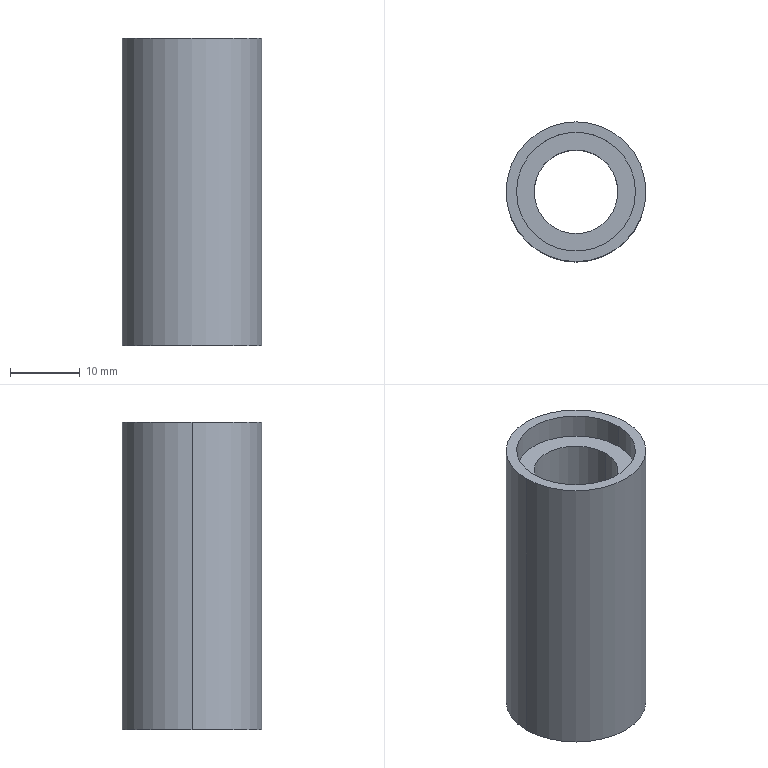Part | STEP file | Shaft 4 PN_0052 | 1 solid | 11 faces | box 20 x 20 x 44 mm | volume 8364 mm3 | cylinder 6 | plane 3 | cone 2 | commonest cylinder face diameters 12 x2 17 x2 20 x2
STEP:
#1=CARTESIAN_POINT('',(0.,0.,0.));
#2=DIRECTION('',(0.,0.,1.));
#3=DIRECTION('',(1.,0.,0.));
#4=AXIS2_PLACEMENT_3D('',#1,#2,#3);
#5=CARTESIAN_POINT('',(10.,0.,0.));
#6=VERTEX_POINT('',#5);
#7=CARTESIAN_POINT('',(-10.,0.,0.));
#8=VERTEX_POINT('',#7);
#9=CARTESIAN_POINT('',(0.,0.,0.));
#10=DIRECTION('',(0.,0.,1.));
#11=DIRECTION('',(1.,0.,0.));
#12=AXIS2_PLACEMENT_3D('',#9,#10,#11);
#13=CIRCLE('',#12,10.);
#14=CARTESIAN_POINT('',(0.,0.,0.));
#15=DIRECTION('',(0.,0.,1.));
#16=DIRECTION('',(1.,0.,0.));
#17=AXIS2_PLACEMENT_3D('',#14,#15,#16);
#18=CYLINDRICAL_SURFACE('',#17,10.);
#19=CARTESIAN_POINT('',(0.,0.));
#20=DIRECTION('',(1.,0.));
#21=VECTOR('',#20,1.);
#22=LINE('',#19,#21);
#23=(GEOMETRIC_REPRESENTATION_CONTEXT(2)PARAMETRIC_REPRESENTATION_CONTEXT()REPRESENTATION_CONTEXT('',''));
#24=DEFINITIONAL_REPRESENTATION('',(#22),#23);
#25=PCURVE('',#18,#24);
#26=CARTESIAN_POINT('',(0.,0.,0.));
#27=DIRECTION('',(0.,0.,-1.));
#28=DIRECTION('',(-1.,0.,0.));
#29=AXIS2_PLACEMENT_3D('',#26,#27,#28);
#30=PLANE('',#29);
#31=CARTESIAN_POINT('',(-10.,0.));
#32=CARTESIAN_POINT('',(-10.,17.321));
#33=CARTESIAN_POINT('',(5.,8.66));
#34=CARTESIAN_POINT('',(20.,0.));
#35=CARTESIAN_POINT('',(5.,-8.66));
#36=CARTESIAN_POINT('',(-10.,-17.321));
#37=CARTESIAN_POINT('',(-10.,0.));
#38=(BOUNDED_CURVE()B_SPLINE_CURVE(2,(#31,#32,#33,#34,#35,#36,#37),.UNSPECIFIED.,.T.,.F.)B_SPLINE_CURVE_WITH_KNOTS((1,2,2,2,2,1),(-2.094,0.,2.094,4.189,6.283,8.378),.UNSPECIFIED.)CURVE()GEOMETRIC_REPRESENTATION_ITEM()RATIONAL_B_SPLINE_CURVE((1.,0.5,1.,0.5,1.,0.5,1.))REPRESENTATION_ITEM(''));
#39=(GEOMETRIC_REPRESENTATION_CONTEXT(2)PARAMETRIC_REPRESENTATION_CONTEXT()REPRESENTATION_CONTEXT('',''));
#40=DEFINITIONAL_REPRESENTATION('',(#38),#39);
#41=PCURVE('',#30,#40);
#42=SURFACE_CURVE('',#13,(#25,#41),.PCURVE_S1.);
#43=EDGE_CURVE('',#6,#8,#42,.T.);
#44=ORIENTED_EDGE('',*,*,#43,.T.);
#45=CARTESIAN_POINT('',(-10.,0.,44.));
#46=VERTEX_POINT('',#45);
#47=CARTESIAN_POINT('',(-10.,0.,0.));
#48=DIRECTION('',(0.,0.,1.));
#49=VECTOR('',#48,1.);
#50=LINE('',#47,#49);
#51=CARTESIAN_POINT('',(3.142,0.));
#52=DIRECTION('',(0.,1.));
#53=VECTOR('',#52,1.);
#54=LINE('',#51,#53);
#55=(GEOMETRIC_REPRESENTATION_CONTEXT(2)PARAMETRIC_REPRESENTATION_CONTEXT()REPRESENTATION_CONTEXT('',''));
#56=DEFINITIONAL_REPRESENTATION('',(#54),#55);
#57=PCURVE('',#18,#56);
#58=CARTESIAN_POINT('',(0.,0.,0.));
#59=DIRECTION('',(0.,0.,1.));
#60=DIRECTION('',(1.,0.,0.));
#61=AXIS2_PLACEMENT_3D('',#58,#59,#60);
#62=CYLINDRICAL_SURFACE('',#61,10.);
#63=CARTESIAN_POINT('',(3.142,0.));
#64=DIRECTION('',(0.,1.));
#65=VECTOR('',#64,1.);
#66=LINE('',#63,#65);
#67=(GEOMETRIC_REPRESENTATION_CONTEXT(2)PARAMETRIC_REPRESENTATION_CONTEXT()REPRESENTATION_CONTEXT('',''));
#68=DEFINITIONAL_REPRESENTATION('',(#66),#67);
#69=PCURVE('',#62,#68);
#70=SURFACE_CURVE('',#50,(#57,#69),.PCURVE_S1.);
#71=EDGE_CURVE('',#8,#46,#70,.T.);
#72=ORIENTED_EDGE('',*,*,#71,.T.);
#73=CARTESIAN_POINT('',(10.,0.,44.));
#74=VERTEX_POINT('',#73);
#75=CARTESIAN_POINT('',(0.,0.,44.));
#76=DIRECTION('',(0.,0.,-1.));
#77=DIRECTION('',(1.,0.,0.));
#78=AXIS2_PLACEMENT_3D('',#75,#76,#77);
#79=CIRCLE('',#78,10.);
#80=CARTESIAN_POINT('',(6.283,44.));
#81=DIRECTION('',(-1.,0.));
#82=VECTOR('',#81,1.);
#83=LINE('',#80,#82);
#84=(GEOMETRIC_REPRESENTATION_CONTEXT(2)PARAMETRIC_REPRESENTATION_CONTEXT()REPRESENTATION_CONTEXT('',''));
#85=DEFINITIONAL_REPRESENTATION('',(#83),#84);
#86=PCURVE('',#18,#85);
#87=CARTESIAN_POINT('',(0.,0.,44.));
#88=DIRECTION('',(0.,0.,-1.));
#89=DIRECTION('',(-1.,0.,0.));
#90=AXIS2_PLACEMENT_3D('',#87,#88,#89);
#91=PLANE('',#90);
#92=CARTESIAN_POINT('',(0.,0.));
#93=DIRECTION('',(-1.,0.));
#94=AXIS2_PLACEMENT_2D('',#92,#93);
#95=CIRCLE('',#94,10.);
#96=(GEOMETRIC_REPRESENTATION_CONTEXT(2)PARAMETRIC_REPRESENTATION_CONTEXT()REPRESENTATION_CONTEXT('',''));
#97=DEFINITIONAL_REPRESENTATION('',(#95),#96);
#98=PCURVE('',#91,#97);
#99=SURFACE_CURVE('',#79,(#86,#98),.PCURVE_S1.);
#100=EDGE_CURVE('',#46,#74,#99,.T.);
#101=ORIENTED_EDGE('',*,*,#100,.T.);
#102=CARTESIAN_POINT('',(10.,0.,0.));
#103=DIRECTION('',(0.,0.,1.));
#104=VECTOR('',#103,1.);
#105=LINE('',#102,#104);
#106=CARTESIAN_POINT('',(0.,0.));
#107=DIRECTION('',(0.,1.));
#108=VECTOR('',#107,1.);
#109=LINE('',#106,#108);
#110=(GEOMETRIC_REPRESENTATION_CONTEXT(2)PARAMETRIC_REPRESENTATION_CONTEXT()REPRESENTATION_CONTEXT('',''));
#111=DEFINITIONAL_REPRESENTATION('',(#109),#110);
#112=PCURVE('',#18,#111);
#113=CARTESIAN_POINT('',(6.283,0.));
#114=DIRECTION('',(0.,1.));
#115=VECTOR('',#114,1.);
#116=LINE('',#113,#115);
#117=(GEOMETRIC_REPRESENTATION_CONTEXT(2)PARAMETRIC_REPRESENTATION_CONTEXT()REPRESENTATION_CONTEXT('',''));
#118=DEFINITIONAL_REPRESENTATION('',(#116),#117);
#119=PCURVE('',#62,#118);
#120=SURFACE_CURVE('',#105,(#112,#119),.PCURVE_S1.);
#121=EDGE_CURVE('',#6,#74,#120,.T.);
#122=ORIENTED_EDGE('',*,*,#121,.F.);
#123=EDGE_LOOP('',(#44,#72,#101,#122));
#124=FACE_BOUND('',#123,.T.);
#125=ADVANCED_FACE('',(#124),#18,.T.);
#126=CARTESIAN_POINT('',(-6.,0.,2.));
#127=VERTEX_POINT('',#126);
#128=CARTESIAN_POINT('',(-8.,0.,-0.000000001));
#129=VERTEX_POINT('',#128);
#130=CARTESIAN_POINT('',(-8.,0.,-0.000000001));
#131=DIRECTION('',(-0.7071,0.,-0.7071));
#132=VECTOR('',#131,1.);
#133=LINE('',#130,#132);
#134=CARTESIAN_POINT('',(0.,0.,-0.000000001));
#135=DIRECTION('',(0.,0.,-1.));
#136=DIRECTION('',(-1.,0.,0.));
#137=AXIS2_PLACEMENT_3D('',#134,#135,#136);
#138=CONICAL_SURFACE('',#137,8.,0.7854);
#139=CARTESIAN_POINT('',(6.283,0.));
#140=DIRECTION('',(0.,1.));
#141=VECTOR('',#140,1.);
#142=LINE('',#139,#141);
#143=(GEOMETRIC_REPRESENTATION_CONTEXT(2)PARAMETRIC_REPRESENTATION_CONTEXT()REPRESENTATION_CONTEXT('',''));
#144=DEFINITIONAL_REPRESENTATION('',(#142),#143);
#145=PCURVE('',#138,#144);
#146=CARTESIAN_POINT('',(0.,0.,-0.000000001));
#147=DIRECTION('',(0.,0.,-1.));
#148=DIRECTION('',(-1.,0.,0.));
#149=AXIS2_PLACEMENT_3D('',#146,#147,#148);
#150=CONICAL_SURFACE('',#149,8.,0.7854);
#151=CARTESIAN_POINT('',(0.,0.));
#152=DIRECTION('',(0.,1.));
#153=VECTOR('',#152,1.);
#154=LINE('',#151,#153);
#155=(GEOMETRIC_REPRESENTATION_CONTEXT(2)PARAMETRIC_REPRESENTATION_CONTEXT()REPRESENTATION_CONTEXT('',''));
#156=DEFINITIONAL_REPRESENTATION('',(#154),#155);
#157=PCURVE('',#150,#156);
#158=SURFACE_CURVE('',#133,(#145,#157),.PCURVE_S1.);
#159=EDGE_CURVE('',#127,#129,#158,.T.);
#160=ORIENTED_EDGE('',*,*,#159,.T.);
#161=CARTESIAN_POINT('',(8.,0.,-0.000000001));
#162=VERTEX_POINT('',#161);
#163=CARTESIAN_POINT('',(0.,0.,-0.000000001));
#164=DIRECTION('',(0.,0.,1.));
#165=DIRECTION('',(-1.,0.,0.));
#166=AXIS2_PLACEMENT_3D('',#163,#164,#165);
#167=CIRCLE('',#166,8.);
#168=CARTESIAN_POINT('',(6.283,0.));
#169=DIRECTION('',(-1.,0.));
#170=VECTOR('',#169,1.);
#171=LINE('',#168,#170);
#172=(GEOMETRIC_REPRESENTATION_CONTEXT(2)PARAMETRIC_REPRESENTATION_CONTEXT()REPRESENTATION_CONTEXT('',''));
#173=DEFINITIONAL_REPRESENTATION('',(#171),#172);
#174=PCURVE('',#138,#173);
#175=CARTESIAN_POINT('',(8.,0.));
#176=CARTESIAN_POINT('',(8.,-13.856));
#177=CARTESIAN_POINT('',(-4.,-6.928));
#178=CARTESIAN_POINT('',(-16.,0.));
#179=CARTESIAN_POINT('',(-4.,6.928));
#180=CARTESIAN_POINT('',(8.,13.856));
#181=CARTESIAN_POINT('',(8.,0.));
#182=(BOUNDED_CURVE()B_SPLINE_CURVE(2,(#175,#176,#177,#178,#179,#180,#181),.UNSPECIFIED.,.T.,.F.)B_SPLINE_CURVE_WITH_KNOTS((1,2,2,2,2,1),(-2.094,0.,2.094,4.189,6.283,8.378),.UNSPECIFIED.)CURVE()GEOMETRIC_REPRESENTATION_ITEM()RATIONAL_B_SPLINE_CURVE((1.,0.5,1.,0.5,1.,0.5,1.))REPRESENTATION_ITEM(''));
#183=(GEOMETRIC_REPRESENTATION_CONTEXT(2)PARAMETRIC_REPRESENTATION_CONTEXT()REPRESENTATION_CONTEXT('',''));
#184=DEFINITIONAL_REPRESENTATION('',(#182),#183);
#185=PCURVE('',#30,#184);
#186=SURFACE_CURVE('',#167,(#174,#185),.PCURVE_S1.);
#187=EDGE_CURVE('',#129,#162,#186,.T.);
#188=ORIENTED_EDGE('',*,*,#187,.T.);
#189=CARTESIAN_POINT('',(6.,0.,2.));
#190=VERTEX_POINT('',#189);
#191=CARTESIAN_POINT('',(8.,0.,-0.000000001));
#192=DIRECTION('',(0.7071,0.,-0.7071));
#193=VECTOR('',#192,1.);
#194=LINE('',#191,#193);
#195=CARTESIAN_POINT('',(3.142,0.));
#196=DIRECTION('',(0.,1.));
#197=VECTOR('',#196,1.);
#198=LINE('',#195,#197);
#199=(GEOMETRIC_REPRESENTATION_CONTEXT(2)PARAMETRIC_REPRESENTATION_CONTEXT()REPRESENTATION_CONTEXT('',''));
#200=DEFINITIONAL_REPRESENTATION('',(#198),#199);
#201=PCURVE('',#138,#200);
#202=CARTESIAN_POINT('',(3.142,0.));
#203=DIRECTION('',(0.,1.));
#204=VECTOR('',#203,1.);
#205=LINE('',#202,#204);
#206=(GEOMETRIC_REPRESENTATION_CONTEXT(2)PARAMETRIC_REPRESENTATION_CONTEXT()REPRESENTATION_CONTEXT('',''));
#207=DEFINITIONAL_REPRESENTATION('',(#205),#206);
#208=PCURVE('',#150,#207);
#209=SURFACE_CURVE('',#194,(#201,#208),.PCURVE_S1.);
#210=EDGE_CURVE('',#190,#162,#209,.T.);
#211=ORIENTED_EDGE('',*,*,#210,.F.);
#212=CARTESIAN_POINT('',(0.,0.,2.));
#213=DIRECTION('',(0.,0.,-1.));
#214=DIRECTION('',(1.,0.,0.));
#215=AXIS2_PLACEMENT_3D('',#212,#213,#214);
#216=CIRCLE('',#215,6.);
#217=CARTESIAN_POINT('',(3.142,-2.));
#218=DIRECTION('',(1.,0.));
#219=VECTOR('',#218,1.);
#220=LINE('',#217,#219);
#221=(GEOMETRIC_REPRESENTATION_CONTEXT(2)PARAMETRIC_REPRESENTATION_CONTEXT()REPRESENTATION_CONTEXT('',''));
#222=DEFINITIONAL_REPRESENTATION('',(#220),#221);
#223=PCURVE('',#138,#222);
#224=CARTESIAN_POINT('',(0.,0.,0.));
#225=DIRECTION('',(0.,0.,1.));
#226=DIRECTION('',(1.,0.,0.));
#227=AXIS2_PLACEMENT_3D('',#224,#225,#226);
#228=CYLINDRICAL_SURFACE('',#227,6.);
#229=CARTESIAN_POINT('',(6.283,2.));
#230=DIRECTION('',(-1.,0.));
#231=VECTOR('',#230,1.);
#232=LINE('',#229,#231);
#233=(GEOMETRIC_REPRESENTATION_CONTEXT(2)PARAMETRIC_REPRESENTATION_CONTEXT()REPRESENTATION_CONTEXT('',''));
#234=DEFINITIONAL_REPRESENTATION('',(#232),#233);
#235=PCURVE('',#228,#234);
#236=SURFACE_CURVE('',#216,(#223,#235),.PCURVE_S1.);
#237=EDGE_CURVE('',#190,#127,#236,.T.);
#238=ORIENTED_EDGE('',*,*,#237,.T.);
#239=EDGE_LOOP('',(#160,#188,#211,#238));
#240=FACE_BOUND('',#239,.F.);
#241=ADVANCED_FACE('',(#240),#138,.F.);
#242=CARTESIAN_POINT('',(-8.5,0.,44.));
#243=VERTEX_POINT('',#242);
#244=CARTESIAN_POINT('',(-8.5,0.,40.5));
#245=VERTEX_POINT('',#244);
#246=CARTESIAN_POINT('',(-8.5,0.,44.));
#247=DIRECTION('',(0.,0.,-1.));
#248=VECTOR('',#247,1.);
#249=LINE('',#246,#248);
#250=CARTESIAN_POINT('',(0.,0.,44.));
#251=DIRECTION('',(0.,0.,-1.));
#252=DIRECTION('',(-1.,0.,0.));
#253=AXIS2_PLACEMENT_3D('',#250,#251,#252);
#254=CYLINDRICAL_SURFACE('',#253,8.5);
#255=CARTESIAN_POINT('',(6.283,0.));
#256=DIRECTION('',(0.,1.));
#257=VECTOR('',#256,1.);
#258=LINE('',#255,#257);
#259=(GEOMETRIC_REPRESENTATION_CONTEXT(2)PARAMETRIC_REPRESENTATION_CONTEXT()REPRESENTATION_CONTEXT('',''));
#260=DEFINITIONAL_REPRESENTATION('',(#258),#259);
#261=PCURVE('',#254,#260);
#262=CARTESIAN_POINT('',(0.,0.,44.));
#263=DIRECTION('',(0.,0.,-1.));
#264=DIRECTION('',(-1.,0.,0.));
#265=AXIS2_PLACEMENT_3D('',#262,#263,#264);
#266=CYLINDRICAL_SURFACE('',#265,8.5);
#267=CARTESIAN_POINT('',(0.,0.));
#268=DIRECTION('',(0.,1.));
#269=VECTOR('',#268,1.);
#270=LINE('',#267,#269);
#271=(GEOMETRIC_REPRESENTATION_CONTEXT(2)PARAMETRIC_REPRESENTATION_CONTEXT()REPRESENTATION_CONTEXT('',''));
#272=DEFINITIONAL_REPRESENTATION('',(#270),#271);
#273=PCURVE('',#266,#272);
#274=SURFACE_CURVE('',#249,(#261,#273),.PCURVE_S1.);
#275=EDGE_CURVE('',#243,#245,#274,.T.);
#276=ORIENTED_EDGE('',*,*,#275,.T.);
#277=CARTESIAN_POINT('',(8.5,0.,40.5));
#278=VERTEX_POINT('',#277);
#279=CARTESIAN_POINT('',(0.,0.,40.5));
#280=DIRECTION('',(0.,0.,1.));
#281=DIRECTION('',(-1.,0.,0.));
#282=AXIS2_PLACEMENT_3D('',#279,#280,#281);
#283=CIRCLE('',#282,8.5);
#284=CARTESIAN_POINT('',(6.283,3.5));
#285=DIRECTION('',(-1.,0.));
#286=VECTOR('',#285,1.);
#287=LINE('',#284,#286);
#288=(GEOMETRIC_REPRESENTATION_CONTEXT(2)PARAMETRIC_REPRESENTATION_CONTEXT()REPRESENTATION_CONTEXT('',''));
#289=DEFINITIONAL_REPRESENTATION('',(#287),#288);
#290=PCURVE('',#254,#289);
#291=CARTESIAN_POINT('',(0.,0.,40.5));
#292=DIRECTION('',(0.,0.,-1.));
#293=DIRECTION('',(-1.,0.,0.));
#294=AXIS2_PLACEMENT_3D('',#291,#292,#293);
#295=PLANE('',#294);
#296=CARTESIAN_POINT('',(8.5,0.));
#297=CARTESIAN_POINT('',(8.5,-14.722));
#298=CARTESIAN_POINT('',(-4.25,-7.361));
#299=CARTESIAN_POINT('',(-17.,0.));
#300=CARTESIAN_POINT('',(-4.25,7.361));
#301=CARTESIAN_POINT('',(8.5,14.722));
#302=CARTESIAN_POINT('',(8.5,0.));
#303=(BOUNDED_CURVE()B_SPLINE_CURVE(2,(#296,#297,#298,#299,#300,#301,#302),.UNSPECIFIED.,.T.,.F.)B_SPLINE_CURVE_WITH_KNOTS((1,2,2,2,2,1),(-2.094,0.,2.094,4.189,6.283,8.378),.UNSPECIFIED.)CURVE()GEOMETRIC_REPRESENTATION_ITEM()RATIONAL_B_SPLINE_CURVE((1.,0.5,1.,0.5,1.,0.5,1.))REPRESENTATION_ITEM(''));
#304=(GEOMETRIC_REPRESENTATION_CONTEXT(2)PARAMETRIC_REPRESENTATION_CONTEXT()REPRESENTATION_CONTEXT('',''));
#305=DEFINITIONAL_REPRESENTATION('',(#303),#304);
#306=PCURVE('',#295,#305);
#307=SURFACE_CURVE('',#283,(#290,#306),.PCURVE_S1.);
#308=EDGE_CURVE('',#245,#278,#307,.T.);
#309=ORIENTED_EDGE('',*,*,#308,.T.);
#310=CARTESIAN_POINT('',(8.5,0.,44.));
#311=VERTEX_POINT('',#310);
#312=CARTESIAN_POINT('',(8.5,0.,44.));
#313=DIRECTION('',(0.,0.,-1.));
#314=VECTOR('',#313,1.);
#315=LINE('',#312,#314);
#316=CARTESIAN_POINT('',(3.142,0.));
#317=DIRECTION('',(0.,1.));
#318=VECTOR('',#317,1.);
#319=LINE('',#316,#318);
#320=(GEOMETRIC_REPRESENTATION_CONTEXT(2)PARAMETRIC_REPRESENTATION_CONTEXT()REPRESENTATION_CONTEXT('',''));
#321=DEFINITIONAL_REPRESENTATION('',(#319),#320);
#322=PCURVE('',#254,#321);
#323=CARTESIAN_POINT('',(3.142,0.));
#324=DIRECTION('',(0.,1.));
#325=VECTOR('',#324,1.);
#326=LINE('',#323,#325);
#327=(GEOMETRIC_REPRESENTATION_CONTEXT(2)PARAMETRIC_REPRESENTATION_CONTEXT()REPRESENTATION_CONTEXT('',''));
#328=DEFINITIONAL_REPRESENTATION('',(#326),#327);
#329=PCURVE('',#266,#328);
#330=SURFACE_CURVE('',#315,(#322,#329),.PCURVE_S1.);
#331=EDGE_CURVE('',#311,#278,#330,.T.);
#332=ORIENTED_EDGE('',*,*,#331,.F.);
#333=CARTESIAN_POINT('',(0.,0.,44.));
#334=DIRECTION('',(0.,0.,1.));
#335=DIRECTION('',(-1.,0.,0.));
#336=AXIS2_PLACEMENT_3D('',#333,#334,#335);
#337=CIRCLE('',#336,8.5);
#338=CARTESIAN_POINT('',(6.283,0.));
#339=DIRECTION('',(-1.,0.));
#340=VECTOR('',#339,1.);
#341=LINE('',#338,#340);
#342=(GEOMETRIC_REPRESENTATION_CONTEXT(2)PARAMETRIC_REPRESENTATION_CONTEXT()REPRESENTATION_CONTEXT('',''));
#343=DEFINITIONAL_REPRESENTATION('',(#341),#342);
#344=PCURVE('',#254,#343);
#345=CARTESIAN_POINT('',(8.5,0.));
#346=CARTESIAN_POINT('',(8.5,-14.722));
#347=CARTESIAN_POINT('',(-4.25,-7.361));
#348=CARTESIAN_POINT('',(-17.,0.));
#349=CARTESIAN_POINT('',(-4.25,7.361));
#350=CARTESIAN_POINT('',(8.5,14.722));
#351=CARTESIAN_POINT('',(8.5,0.));
#352=(BOUNDED_CURVE()B_SPLINE_CURVE(2,(#345,#346,#347,#348,#349,#350,#351),.UNSPECIFIED.,.T.,.F.)B_SPLINE_CURVE_WITH_KNOTS((1,2,2,2,2,1),(-2.094,0.,2.094,4.189,6.283,8.378),.UNSPECIFIED.)CURVE()GEOMETRIC_REPRESENTATION_ITEM()RATIONAL_B_SPLINE_CURVE((1.,0.5,1.,0.5,1.,0.5,1.))REPRESENTATION_ITEM(''));
#353=(GEOMETRIC_REPRESENTATION_CONTEXT(2)PARAMETRIC_REPRESENTATION_CONTEXT()REPRESENTATION_CONTEXT('',''));
#354=DEFINITIONAL_REPRESENTATION('',(#352),#353);
#355=PCURVE('',#91,#354);
#356=SURFACE_CURVE('',#337,(#344,#355),.PCURVE_S1.);
#357=EDGE_CURVE('',#243,#311,#356,.T.);
#358=ORIENTED_EDGE('',*,*,#357,.F.);
#359=EDGE_LOOP('',(#276,#309,#332,#358));
#360=FACE_BOUND('',#359,.F.);
#361=ADVANCED_FACE('',(#360),#254,.F.);
#362=CARTESIAN_POINT('',(6.,0.,40.5));
#363=VERTEX_POINT('',#362);
#364=CARTESIAN_POINT('',(6.,0.,0.));
#365=DIRECTION('',(0.,0.,1.));
#366=VECTOR('',#365,1.);
#367=LINE('',#364,#366);
#368=CARTESIAN_POINT('',(6.283,0.));
#369=DIRECTION('',(0.,1.));
#370=VECTOR('',#369,1.);
#371=LINE('',#368,#370);
#372=(GEOMETRIC_REPRESENTATION_CONTEXT(2)PARAMETRIC_REPRESENTATION_CONTEXT()REPRESENTATION_CONTEXT('',''));
#373=DEFINITIONAL_REPRESENTATION('',(#371),#372);
#374=PCURVE('',#228,#373);
#375=CARTESIAN_POINT('',(0.,0.,0.));
#376=DIRECTION('',(0.,0.,1.));
#377=DIRECTION('',(1.,0.,0.));
#378=AXIS2_PLACEMENT_3D('',#375,#376,#377);
#379=CYLINDRICAL_SURFACE('',#378,6.);
#380=CARTESIAN_POINT('',(0.,0.));
#381=DIRECTION('',(0.,1.));
#382=VECTOR('',#381,1.);
#383=LINE('',#380,#382);
#384=(GEOMETRIC_REPRESENTATION_CONTEXT(2)PARAMETRIC_REPRESENTATION_CONTEXT()REPRESENTATION_CONTEXT('',''));
#385=DEFINITIONAL_REPRESENTATION('',(#383),#384);
#386=PCURVE('',#379,#385);
#387=SURFACE_CURVE('',#367,(#374,#386),.PCURVE_S1.);
#388=EDGE_CURVE('',#190,#363,#387,.T.);
#389=ORIENTED_EDGE('',*,*,#388,.T.);
#390=CARTESIAN_POINT('',(-6.,0.,40.5));
#391=VERTEX_POINT('',#390);
#392=CARTESIAN_POINT('',(0.,0.,40.5));
#393=DIRECTION('',(0.,0.,-1.));
#394=DIRECTION('',(1.,0.,0.));
#395=AXIS2_PLACEMENT_3D('',#392,#393,#394);
#396=CIRCLE('',#395,6.);
#397=CARTESIAN_POINT('',(6.283,40.5));
#398=DIRECTION('',(-1.,0.));
#399=VECTOR('',#398,1.);
#400=LINE('',#397,#399);
#401=(GEOMETRIC_REPRESENTATION_CONTEXT(2)PARAMETRIC_REPRESENTATION_CONTEXT()REPRESENTATION_CONTEXT('',''));
#402=DEFINITIONAL_REPRESENTATION('',(#400),#401);
#403=PCURVE('',#228,#402);
#404=CARTESIAN_POINT('',(0.,0.));
#405=DIRECTION('',(-1.,0.));
#406=AXIS2_PLACEMENT_2D('',#404,#405);
#407=CIRCLE('',#406,6.);
#408=(GEOMETRIC_REPRESENTATION_CONTEXT(2)PARAMETRIC_REPRESENTATION_CONTEXT()REPRESENTATION_CONTEXT('',''));
#409=DEFINITIONAL_REPRESENTATION('',(#407),#408);
#410=PCURVE('',#295,#409);
#411=SURFACE_CURVE('',#396,(#403,#410),.PCURVE_S1.);
#412=EDGE_CURVE('',#363,#391,#411,.T.);
#413=ORIENTED_EDGE('',*,*,#412,.T.);
#414=CARTESIAN_POINT('',(-6.,0.,0.));
#415=DIRECTION('',(0.,0.,1.));
#416=VECTOR('',#415,1.);
#417=LINE('',#414,#416);
#418=CARTESIAN_POINT('',(3.142,0.));
#419=DIRECTION('',(0.,1.));
#420=VECTOR('',#419,1.);
#421=LINE('',#418,#420);
#422=(GEOMETRIC_REPRESENTATION_CONTEXT(2)PARAMETRIC_REPRESENTATION_CONTEXT()REPRESENTATION_CONTEXT('',''));
#423=DEFINITIONAL_REPRESENTATION('',(#421),#422);
#424=PCURVE('',#228,#423);
#425=CARTESIAN_POINT('',(3.142,0.));
#426=DIRECTION('',(0.,1.));
#427=VECTOR('',#426,1.);
#428=LINE('',#425,#427);
#429=(GEOMETRIC_REPRESENTATION_CONTEXT(2)PARAMETRIC_REPRESENTATION_CONTEXT()REPRESENTATION_CONTEXT('',''));
#430=DEFINITIONAL_REPRESENTATION('',(#428),#429);
#431=PCURVE('',#379,#430);
#432=SURFACE_CURVE('',#417,(#424,#431),.PCURVE_S1.);
#433=EDGE_CURVE('',#127,#391,#432,.T.);
#434=ORIENTED_EDGE('',*,*,#433,.F.);
#435=ORIENTED_EDGE('',*,*,#237,.F.);
#436=EDGE_LOOP('',(#389,#413,#434,#435));
#437=FACE_BOUND('',#436,.F.);
#438=ADVANCED_FACE('',(#437),#228,.F.);
#439=ORIENTED_EDGE('',*,*,#71,.F.);
#440=CARTESIAN_POINT('',(0.,0.,0.));
#441=DIRECTION('',(0.,0.,1.));
#442=DIRECTION('',(1.,0.,0.));
#443=AXIS2_PLACEMENT_3D('',#440,#441,#442);
#444=CIRCLE('',#443,10.);
#445=CARTESIAN_POINT('',(0.,0.));
#446=DIRECTION('',(1.,0.));
#447=VECTOR('',#446,1.);
#448=LINE('',#445,#447);
#449=(GEOMETRIC_REPRESENTATION_CONTEXT(2)PARAMETRIC_REPRESENTATION_CONTEXT()REPRESENTATION_CONTEXT('',''));
#450=DEFINITIONAL_REPRESENTATION('',(#448),#449);
#451=PCURVE('',#62,#450);
#452=CARTESIAN_POINT('',(-10.,0.));
#453=CARTESIAN_POINT('',(-10.,17.321));
#454=CARTESIAN_POINT('',(5.,8.66));
#455=CARTESIAN_POINT('',(20.,0.));
#456=CARTESIAN_POINT('',(5.,-8.66));
#457=CARTESIAN_POINT('',(-10.,-17.321));
#458=CARTESIAN_POINT('',(-10.,0.));
#459=(BOUNDED_CURVE()B_SPLINE_CURVE(2,(#452,#453,#454,#455,#456,#457,#458),.UNSPECIFIED.,.T.,.F.)B_SPLINE_CURVE_WITH_KNOTS((1,2,2,2,2,1),(-2.094,0.,2.094,4.189,6.283,8.378),.UNSPECIFIED.)CURVE()GEOMETRIC_REPRESENTATION_ITEM()RATIONAL_B_SPLINE_CURVE((1.,0.5,1.,0.5,1.,0.5,1.))REPRESENTATION_ITEM(''));
#460=(GEOMETRIC_REPRESENTATION_CONTEXT(2)PARAMETRIC_REPRESENTATION_CONTEXT()REPRESENTATION_CONTEXT('',''));
#461=DEFINITIONAL_REPRESENTATION('',(#459),#460);
#462=PCURVE('',#30,#461);
#463=SURFACE_CURVE('',#444,(#451,#462),.PCURVE_S1.);
#464=EDGE_CURVE('',#8,#6,#463,.T.);
#465=ORIENTED_EDGE('',*,*,#464,.T.);
#466=ORIENTED_EDGE('',*,*,#121,.T.);
#467=CARTESIAN_POINT('',(0.,0.,44.));
#468=DIRECTION('',(0.,0.,-1.));
#469=DIRECTION('',(1.,0.,0.));
#470=AXIS2_PLACEMENT_3D('',#467,#468,#469);
#471=CIRCLE('',#470,10.);
#472=CARTESIAN_POINT('',(6.283,44.));
#473=DIRECTION('',(-1.,0.));
#474=VECTOR('',#473,1.);
#475=LINE('',#472,#474);
#476=(GEOMETRIC_REPRESENTATION_CONTEXT(2)PARAMETRIC_REPRESENTATION_CONTEXT()REPRESENTATION_CONTEXT('',''));
#477=DEFINITIONAL_REPRESENTATION('',(#475),#476);
#478=PCURVE('',#62,#477);
#479=CARTESIAN_POINT('',(0.,0.));
#480=DIRECTION('',(-1.,0.));
#481=AXIS2_PLACEMENT_2D('',#479,#480);
#482=CIRCLE('',#481,10.);
#483=(GEOMETRIC_REPRESENTATION_CONTEXT(2)PARAMETRIC_REPRESENTATION_CONTEXT()REPRESENTATION_CONTEXT('',''));
#484=DEFINITIONAL_REPRESENTATION('',(#482),#483);
#485=PCURVE('',#91,#484);
#486=SURFACE_CURVE('',#471,(#478,#485),.PCURVE_S1.);
#487=EDGE_CURVE('',#74,#46,#486,.T.);
#488=ORIENTED_EDGE('',*,*,#487,.T.);
#489=EDGE_LOOP('',(#439,#465,#466,#488));
#490=FACE_BOUND('',#489,.T.);
#491=ADVANCED_FACE('',(#490),#62,.T.);
#492=ORIENTED_EDGE('',*,*,#187,.T.);
#493=CARTESIAN_POINT('',(0.,0.,-0.000000001));
#494=DIRECTION('',(0.,0.,1.));
#495=DIRECTION('',(-1.,0.,0.));
#496=AXIS2_PLACEMENT_3D('',#493,#494,#495);
#497=CIRCLE('',#496,8.);
#498=CARTESIAN_POINT('',(8.,0.));
#499=CARTESIAN_POINT('',(8.,-13.856));
#500=CARTESIAN_POINT('',(-4.,-6.928));
#501=CARTESIAN_POINT('',(-16.,0.));
#502=CARTESIAN_POINT('',(-4.,6.928));
#503=CARTESIAN_POINT('',(8.,13.856));
#504=CARTESIAN_POINT('',(8.,0.));
#505=(BOUNDED_CURVE()B_SPLINE_CURVE(2,(#498,#499,#500,#501,#502,#503,#504),.UNSPECIFIED.,.T.,.F.)B_SPLINE_CURVE_WITH_KNOTS((1,2,2,2,2,1),(-2.094,0.,2.094,4.189,6.283,8.378),.UNSPECIFIED.)CURVE()GEOMETRIC_REPRESENTATION_ITEM()RATIONAL_B_SPLINE_CURVE((1.,0.5,1.,0.5,1.,0.5,1.))REPRESENTATION_ITEM(''));
#506=(GEOMETRIC_REPRESENTATION_CONTEXT(2)PARAMETRIC_REPRESENTATION_CONTEXT()REPRESENTATION_CONTEXT('',''));
#507=DEFINITIONAL_REPRESENTATION('',(#505),#506);
#508=PCURVE('',#30,#507);
#509=CARTESIAN_POINT('',(6.283,0.));
#510=DIRECTION('',(-1.,0.));
#511=VECTOR('',#510,1.);
#512=LINE('',#509,#511);
#513=(GEOMETRIC_REPRESENTATION_CONTEXT(2)PARAMETRIC_REPRESENTATION_CONTEXT()REPRESENTATION_CONTEXT('',''));
#514=DEFINITIONAL_REPRESENTATION('',(#512),#513);
#515=PCURVE('',#150,#514);
#516=SURFACE_CURVE('',#497,(#508,#515),.PCURVE_S1.);
#517=EDGE_CURVE('',#162,#129,#516,.T.);
#518=ORIENTED_EDGE('',*,*,#517,.T.);
#519=EDGE_LOOP('',(#492,#518));
#520=FACE_BOUND('',#519,.T.);
#521=ORIENTED_EDGE('',*,*,#43,.F.);
#522=ORIENTED_EDGE('',*,*,#464,.F.);
#523=EDGE_LOOP('',(#521,#522));
#524=FACE_BOUND('',#523,.T.);
#525=ADVANCED_FACE('',(#520,#524),#30,.T.);
#526=ORIENTED_EDGE('',*,*,#357,.F.);
#527=CARTESIAN_POINT('',(0.,0.,44.));
#528=DIRECTION('',(0.,0.,1.));
#529=DIRECTION('',(-1.,0.,0.));
#530=AXIS2_PLACEMENT_3D('',#527,#528,#529);
#531=CIRCLE('',#530,8.5);
#532=CARTESIAN_POINT('',(8.5,0.));
#533=CARTESIAN_POINT('',(8.5,-14.722));
#534=CARTESIAN_POINT('',(-4.25,-7.361));
#535=CARTESIAN_POINT('',(-17.,0.));
#536=CARTESIAN_POINT('',(-4.25,7.361));
#537=CARTESIAN_POINT('',(8.5,14.722));
#538=CARTESIAN_POINT('',(8.5,0.));
#539=(BOUNDED_CURVE()B_SPLINE_CURVE(2,(#532,#533,#534,#535,#536,#537,#538),.UNSPECIFIED.,.T.,.F.)B_SPLINE_CURVE_WITH_KNOTS((1,2,2,2,2,1),(-2.094,0.,2.094,4.189,6.283,8.378),.UNSPECIFIED.)CURVE()GEOMETRIC_REPRESENTATION_ITEM()RATIONAL_B_SPLINE_CURVE((1.,0.5,1.,0.5,1.,0.5,1.))REPRESENTATION_ITEM(''));
#540=(GEOMETRIC_REPRESENTATION_CONTEXT(2)PARAMETRIC_REPRESENTATION_CONTEXT()REPRESENTATION_CONTEXT('',''));
#541=DEFINITIONAL_REPRESENTATION('',(#539),#540);
#542=PCURVE('',#91,#541);
#543=CARTESIAN_POINT('',(6.283,0.));
#544=DIRECTION('',(-1.,0.));
#545=VECTOR('',#544,1.);
#546=LINE('',#543,#545);
#547=(GEOMETRIC_REPRESENTATION_CONTEXT(2)PARAMETRIC_REPRESENTATION_CONTEXT()REPRESENTATION_CONTEXT('',''));
#548=DEFINITIONAL_REPRESENTATION('',(#546),#547);
#549=PCURVE('',#266,#548);
#550=SURFACE_CURVE('',#531,(#542,#549),.PCURVE_S1.);
#551=EDGE_CURVE('',#311,#243,#550,.T.);
#552=ORIENTED_EDGE('',*,*,#551,.F.);
#553=EDGE_LOOP('',(#526,#552));
#554=FACE_BOUND('',#553,.T.);
#555=ORIENTED_EDGE('',*,*,#487,.F.);
#556=ORIENTED_EDGE('',*,*,#100,.F.);
#557=EDGE_LOOP('',(#555,#556));
#558=FACE_BOUND('',#557,.T.);
#559=ADVANCED_FACE('',(#554,#558),#91,.F.);
#560=ORIENTED_EDGE('',*,*,#517,.T.);
#561=ORIENTED_EDGE('',*,*,#159,.F.);
#562=CARTESIAN_POINT('',(0.,0.,2.));
#563=DIRECTION('',(0.,0.,-1.));
#564=DIRECTION('',(1.,0.,0.));
#565=AXIS2_PLACEMENT_3D('',#562,#563,#564);
#566=CIRCLE('',#565,6.);
#567=CARTESIAN_POINT('',(-3.142,-2.));
#568=DIRECTION('',(1.,0.));
#569=VECTOR('',#568,1.);
#570=LINE('',#567,#569);
#571=(GEOMETRIC_REPRESENTATION_CONTEXT(2)PARAMETRIC_REPRESENTATION_CONTEXT()REPRESENTATION_CONTEXT('',''));
#572=DEFINITIONAL_REPRESENTATION('',(#570),#571);
#573=PCURVE('',#150,#572);
#574=CARTESIAN_POINT('',(6.283,2.));
#575=DIRECTION('',(-1.,0.));
#576=VECTOR('',#575,1.);
#577=LINE('',#574,#576);
#578=(GEOMETRIC_REPRESENTATION_CONTEXT(2)PARAMETRIC_REPRESENTATION_CONTEXT()REPRESENTATION_CONTEXT('',''));
#579=DEFINITIONAL_REPRESENTATION('',(#577),#578);
#580=PCURVE('',#379,#579);
#581=SURFACE_CURVE('',#566,(#573,#580),.PCURVE_S1.);
#582=EDGE_CURVE('',#127,#190,#581,.T.);
#583=ORIENTED_EDGE('',*,*,#582,.T.);
#584=ORIENTED_EDGE('',*,*,#210,.T.);
#585=EDGE_LOOP('',(#560,#561,#583,#584));
#586=FACE_BOUND('',#585,.F.);
#587=ADVANCED_FACE('',(#586),#150,.F.);
#588=CARTESIAN_POINT('',(0.,0.,40.5));
#589=DIRECTION('',(0.,0.,1.));
#590=DIRECTION('',(-1.,0.,0.));
#591=AXIS2_PLACEMENT_3D('',#588,#589,#590);
#592=CIRCLE('',#591,8.5);
#593=CARTESIAN_POINT('',(6.283,3.5));
#594=DIRECTION('',(-1.,0.));
#595=VECTOR('',#594,1.);
#596=LINE('',#593,#595);
#597=(GEOMETRIC_REPRESENTATION_CONTEXT(2)PARAMETRIC_REPRESENTATION_CONTEXT()REPRESENTATION_CONTEXT('',''));
#598=DEFINITIONAL_REPRESENTATION('',(#596),#597);
#599=PCURVE('',#266,#598);
#600=CARTESIAN_POINT('',(8.5,0.));
#601=CARTESIAN_POINT('',(8.5,-14.722));
#602=CARTESIAN_POINT('',(-4.25,-7.361));
#603=CARTESIAN_POINT('',(-17.,0.));
#604=CARTESIAN_POINT('',(-4.25,7.361));
#605=CARTESIAN_POINT('',(8.5,14.722));
#606=CARTESIAN_POINT('',(8.5,0.));
#607=(BOUNDED_CURVE()B_SPLINE_CURVE(2,(#600,#601,#602,#603,#604,#605,#606),.UNSPECIFIED.,.T.,.F.)B_SPLINE_CURVE_WITH_KNOTS((1,2,2,2,2,1),(-2.094,0.,2.094,4.189,6.283,8.378),.UNSPECIFIED.)CURVE()GEOMETRIC_REPRESENTATION_ITEM()RATIONAL_B_SPLINE_CURVE((1.,0.5,1.,0.5,1.,0.5,1.))REPRESENTATION_ITEM(''));
#608=(GEOMETRIC_REPRESENTATION_CONTEXT(2)PARAMETRIC_REPRESENTATION_CONTEXT()REPRESENTATION_CONTEXT('',''));
#609=DEFINITIONAL_REPRESENTATION('',(#607),#608);
#610=PCURVE('',#295,#609);
#611=SURFACE_CURVE('',#592,(#599,#610),.PCURVE_S1.);
#612=EDGE_CURVE('',#278,#245,#611,.T.);
#613=ORIENTED_EDGE('',*,*,#612,.T.);
#614=ORIENTED_EDGE('',*,*,#275,.F.);
#615=ORIENTED_EDGE('',*,*,#551,.F.);
#616=ORIENTED_EDGE('',*,*,#331,.T.);
#617=EDGE_LOOP('',(#613,#614,#615,#616));
#618=FACE_BOUND('',#617,.F.);
#619=ADVANCED_FACE('',(#618),#266,.F.);
#620=CARTESIAN_POINT('',(0.,0.,40.5));
#621=DIRECTION('',(0.,0.,-1.));
#622=DIRECTION('',(1.,0.,0.));
#623=AXIS2_PLACEMENT_3D('',#620,#621,#622);
#624=CIRCLE('',#623,6.);
#625=CARTESIAN_POINT('',(6.283,40.5));
#626=DIRECTION('',(-1.,0.));
#627=VECTOR('',#626,1.);
#628=LINE('',#625,#627);
#629=(GEOMETRIC_REPRESENTATION_CONTEXT(2)PARAMETRIC_REPRESENTATION_CONTEXT()REPRESENTATION_CONTEXT('',''));
#630=DEFINITIONAL_REPRESENTATION('',(#628),#629);
#631=PCURVE('',#379,#630);
#632=CARTESIAN_POINT('',(0.,0.));
#633=DIRECTION('',(-1.,0.));
#634=AXIS2_PLACEMENT_2D('',#632,#633);
#635=CIRCLE('',#634,6.);
#636=(GEOMETRIC_REPRESENTATION_CONTEXT(2)PARAMETRIC_REPRESENTATION_CONTEXT()REPRESENTATION_CONTEXT('',''));
#637=DEFINITIONAL_REPRESENTATION('',(#635),#636);
#638=PCURVE('',#295,#637);
#639=SURFACE_CURVE('',#624,(#631,#638),.PCURVE_S1.);
#640=EDGE_CURVE('',#391,#363,#639,.T.);
#641=ORIENTED_EDGE('',*,*,#640,.T.);
#642=ORIENTED_EDGE('',*,*,#388,.F.);
#643=ORIENTED_EDGE('',*,*,#582,.F.);
#644=ORIENTED_EDGE('',*,*,#433,.T.);
#645=EDGE_LOOP('',(#641,#642,#643,#644));
#646=FACE_BOUND('',#645,.F.);
#647=ADVANCED_FACE('',(#646),#379,.F.);
#648=ORIENTED_EDGE('',*,*,#412,.T.);
#649=ORIENTED_EDGE('',*,*,#640,.T.);
#650=EDGE_LOOP('',(#648,#649));
#651=FACE_BOUND('',#650,.T.);
#652=ORIENTED_EDGE('',*,*,#308,.T.);
#653=ORIENTED_EDGE('',*,*,#612,.T.);
#654=EDGE_LOOP('',(#652,#653));
#655=FACE_BOUND('',#654,.T.);
#656=ADVANCED_FACE('',(#651,#655),#295,.F.);
#657=CLOSED_SHELL('',(#125,#241,#361,#438,#491,#525,#559,#587,#619,#647,#656));
#658=MANIFOLD_SOLID_BREP('',#657);
#659=(LENGTH_UNIT()NAMED_UNIT(*)SI_UNIT(.MILLI.,.METRE.));
#660=UNCERTAINTY_MEASURE_WITH_UNIT(LENGTH_MEASURE(0.0000001),#659,'','');
#661=(NAMED_UNIT(*)PLANE_ANGLE_UNIT()SI_UNIT($,.RADIAN.));
#662=(NAMED_UNIT(*)SI_UNIT($,.STERADIAN.)SOLID_ANGLE_UNIT());
#663=(GEOMETRIC_REPRESENTATION_CONTEXT(3)GLOBAL_UNCERTAINTY_ASSIGNED_CONTEXT((#660))GLOBAL_UNIT_ASSIGNED_CONTEXT((#659,#661,#662))REPRESENTATION_CONTEXT('',''));
#664=ADVANCED_BREP_SHAPE_REPRESENTATION('',(#4,#658),#663);